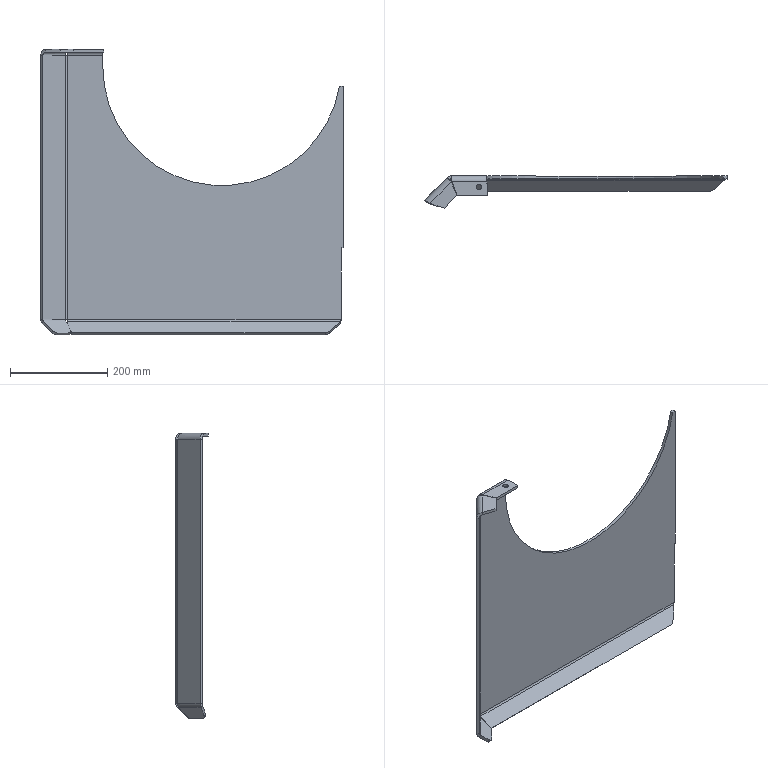Part | SolidWorks | features ICE 3, EdgeFlange 2, SMBaseFlange 2, Fillet 1, FlatPattern 1, SheetMetal 1 | 1 solid | 60 faces | box 622 x 66.558 x 586.477 mm | volume 1620152 mm3 | plane 40 | cylinder 15 | spline 5 | commonest cylinder face diameters 12 x5 24 x5 11 x2 20 x2 490 x1